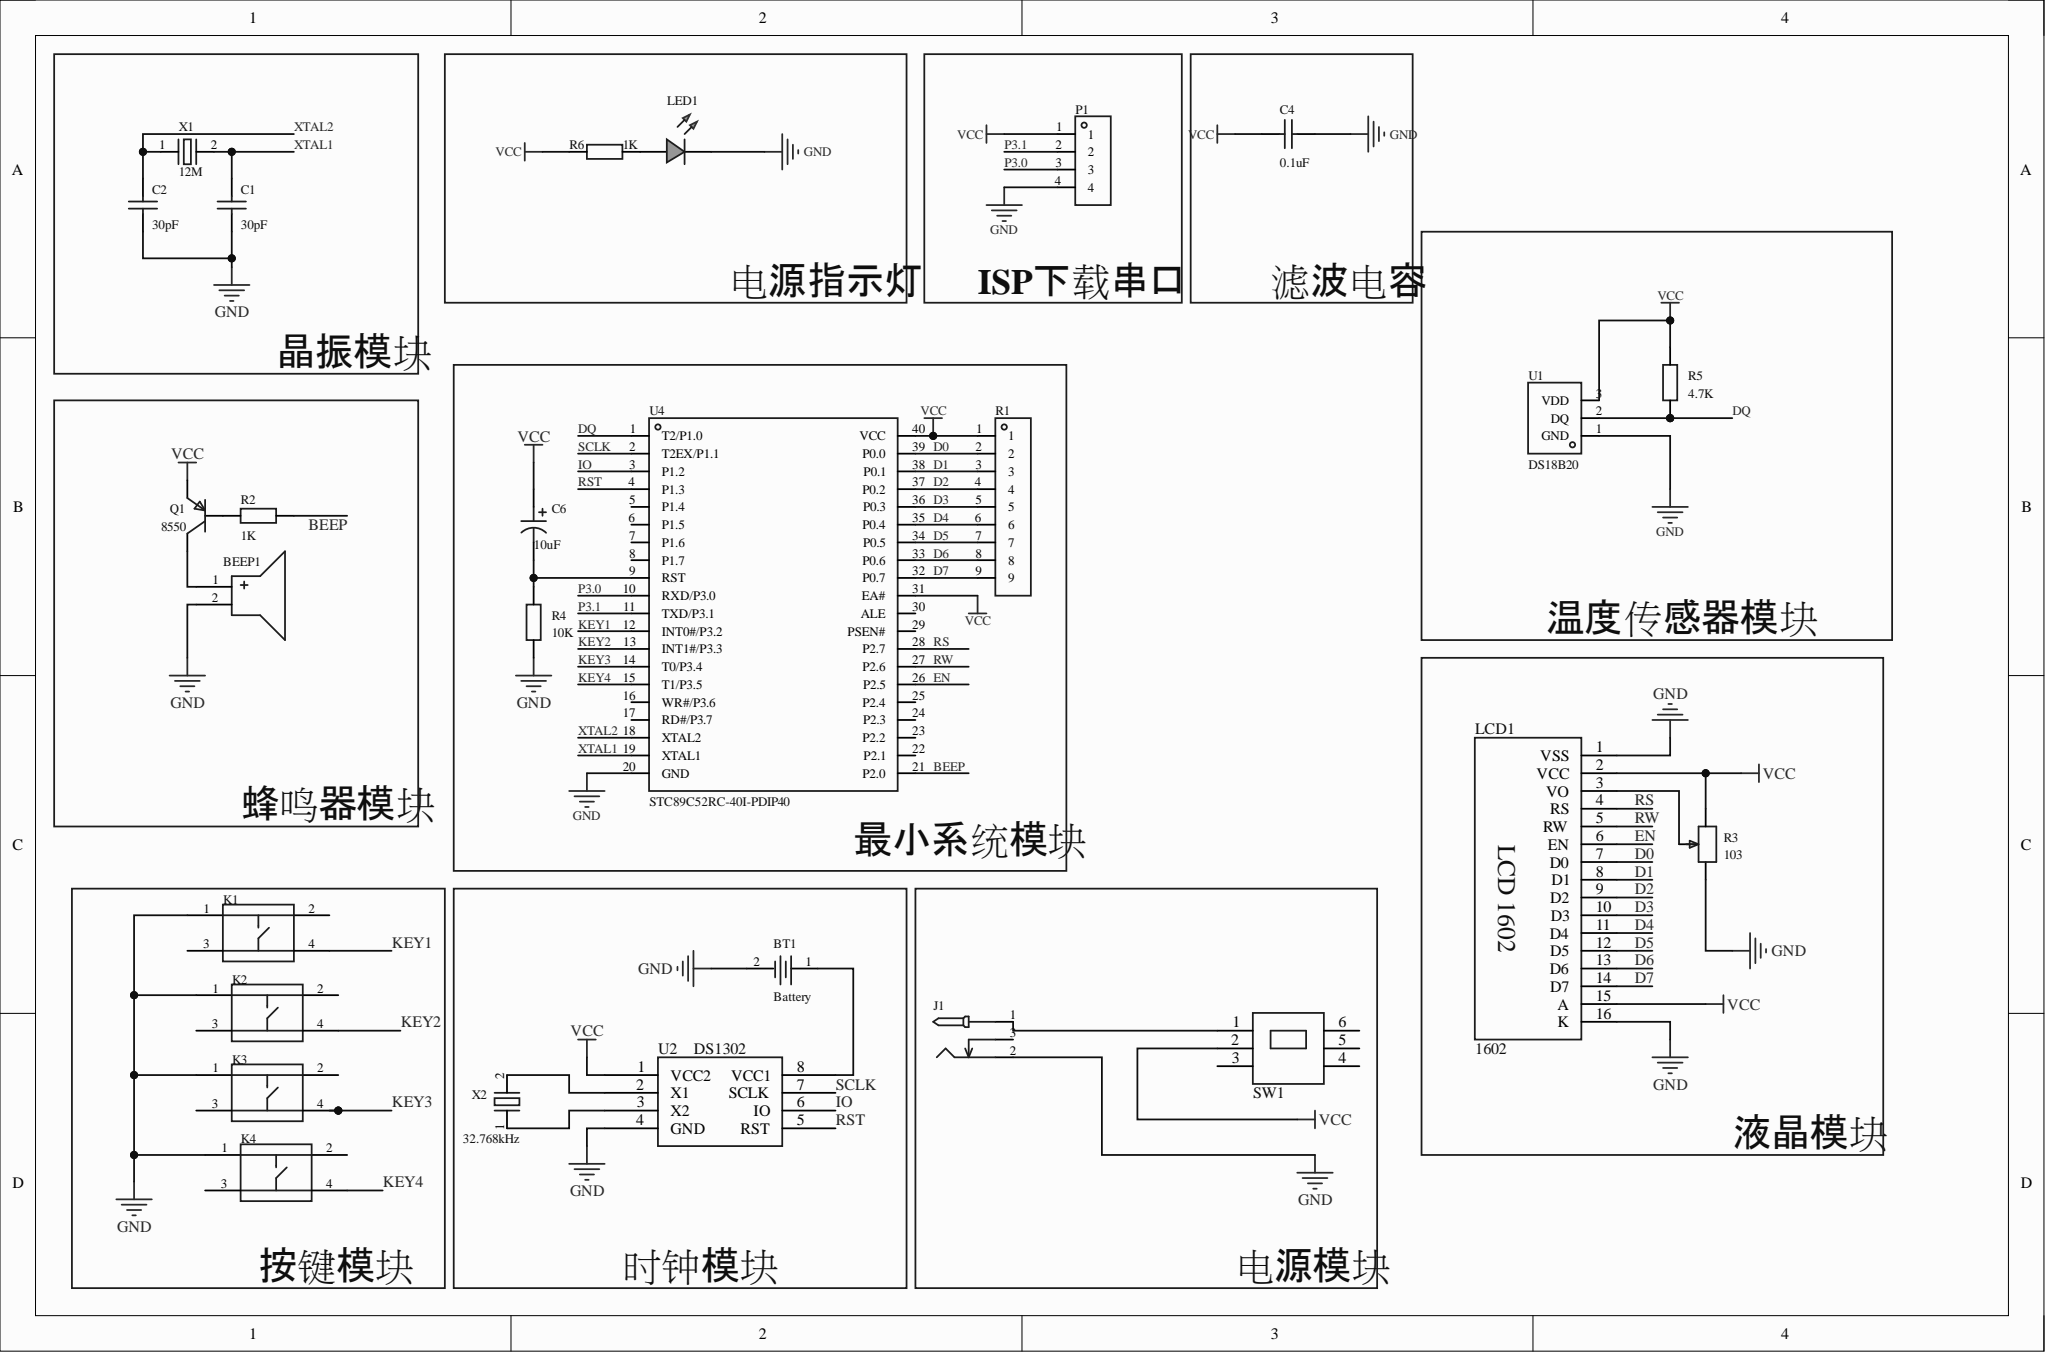Circuit board | Altium Designer | 27 parts | 35 nets
Bill of materials:
Comment,Description,Designator,Footprint,LibRef,Quantity
"","","BEEP1","BUZ-TH_BD12.0-P7.60-D0.6-FD","BZ-D12-L7_6","1"
"Battery","","BT1","BAT-TH_CR2032","Q&J CR2032 20-6*9_C9900112302","1"
"30pF","容值:-;额定电压:-;温度系数:-;","C1, C2","CAP-TH_L5.0-W4.0-P5.00-D1.0","瓷片电容47PF 3KV","2"
"0.1uF","容值:-;额定电压:-;温度系数:-;","C4","CAP-TH_L5.0-W4.0-P5.00-D1.0","瓷片电容47PF 3KV","1"
"10uF","","C6","CAP-TH_BD5.0-P2.00-D0.6-FD","10uF/25V-C5X11DIP","1"
"","","J1","DC-005_2.5","DC-005_2.5","1"
"","电路结构:单刀单掷;按钮形状:圆形按钮;作用力:2.5N;安装方式:直插;开关长度:6mm;开关宽度:6mm;开关高度:5mm;触点电流:50mA;额定电压:12V;带灯:-;工作寿命:10万次;","K1, K2, K3, K4","KEY-TH_4P-L6.0-W6.0-P4.50-LS6.50","K2-1102DP-C4SW-04","4"
"1602","","LCD1","HDR-M-2.54_1X16","1602_1","1"
"","","LED1","LED-TH_5mm","LED_TH-G_5mm","1"
"","","P1","HDR-TH_4P-P2.54-V-M","HDR-M_2.54_1x4P","1"
"8550","","Q1","S8550P_TO-92","S8550_TO_PNP","1"
"","","R1","SIP-9_L22.3-W3.2-P2.54_KA2284-SIP-9","HDR-M_2.54-1x9P","1"
"1K","","R2, R6","Res_1/4W","Res_AXIAL-1/4W","2"
"103","","R3","RES-ADJ-SMD_RM065-V1","RM065-V1-103","1"
"10K","","R4","Res_1/4W","Res_AXIAL-1/4W","1"
"4.7K","","R5","Res_1/4W","Res_AXIAL-1/4W","1"
"SWT","","SW1","SW-TH_6P-L8.5-W8.5-P2.50-LS5.5-BL-2","SWT_1","1"
"DS18B20","检测温度:-55℃~+125℃;精度:±0.4℃;接口类型:单总线;","U1","TO-92-3_L4.5-W3.5-P1.27-L","DS18B20","1"
"DS1302","","U2","DIP-8_L10.9-W6.4-P2.54-LS7.6-BL","DS1302","1"
"STC89C52RC-40I-PDIP40","CPU内核:51家族;CPU最大主频:-;","U4","DIP-40_L52.0-W13.7-P2.54-LS15.2-BL","STC89C52RC-40I-PDIP40","1"
"12M","晶振类型:直插晶振;频率:16MHz;常温频差:±20ppm;负载电容:12pF;频率稳定度:±30ppm;","X1","HC-49S_L11.5-W4.7-P4.88","SWXSBBCVE0-16","1"
"32.768kHz","频率:32.768kHz;常温频差:±20ppm;外接负载电容:12.5pF;频率稳定度(全温):-;","X2","XTAL2","AB15T-32.768KHZ","1"
Netlist (Protel format):
[
BEEP1
BUZ-TH_BD12.0-P7.60-D0.6-FD




]
[
BT1
BAT-TH_CR2032
Battery



]
[
C1
CAP-TH_L5.0-W4.0-P5.00-D1.0
30pF



]
[
C2
CAP-TH_L5.0-W4.0-P5.00-D1.0
30pF



]
[
C4
CAP-TH_L5.0-W4.0-P5.00-D1.0
0.1uF



]
[
C6
CAP-TH_BD5.0-P2.00-D0.6-FD
10uF



]
[
J1
DC-005_2.5




]
[
K1
KEY-TH_4P-L6.0-W6.0-P4.50-LS6.50




]
[
K2
KEY-TH_4P-L6.0-W6.0-P4.50-LS6.50




]
[
K3
KEY-TH_4P-L6.0-W6.0-P4.50-LS6.50




]
[
K4
KEY-TH_4P-L6.0-W6.0-P4.50-LS6.50




]
[
LCD1
HDR-M-2.54_1X16
1602



]
[
LED1
LED-TH_5mm




]
[
P1
HDR-TH_4P-P2.54-V-M




]
[
Q1
S8550P_TO-92
8550



]
[
R1
SIP-9_L22.3-W3.2-P2.54_KA2284-SIP-9




]
[
R2
Res_1/4W
1K



]
[
R3
RES-ADJ-SMD_RM065-V1
103



]
[
R4
Res_1/4W
10K



]
[
R5
Res_1/4W
4.7K



]
[
R6
Res_1/4W
1K



]
[
SW1
SW-TH_6P-L8.5-W8.5-P2.50-LS5.5-BL-2
SWT



]
[
U1
TO-92-3_L4.5-W3.5-P1.27-L
DS18B20



]
[
U2
DIP-8_L10.9-W6.4-P2.54-LS7.6-BL
DS1302



]
[
U4
DIP-40_L52.0-W13.7-P2.54-LS15.2-BL
STC89C52RC-40I-PDIP40



]
[
X1
HC-49S_L11.5-W4.7-P4.88
12M



]
[
X2
XTAL2
32.768kHz



]
(
XTAL2
C2-2
U4-18
X1-1
)
(
XTAL1
C1-2
U4-19
X1-2
)
(
VCC
C4-1
C6-1
LCD1-2
LCD1-15
P1-1
Q1-1
R1-1
R3-3
R5-2
R6-1
SW1-2
U1-3
U2-1
U4-31
U4-40
)
(
SCLK
U2-7
U4-2
)
(
RW
LCD1-5
U4-27
)
(
RST
U2-5
U4-4
)
(
RS
LCD1-4
U4-28
)
(
P3.1
P1-2
U4-11
)
(
P3.0
P1-3
U4-10
)
(
NetU2_3
U2-3
X2-1
)
(
NetU2_2
U2-2
X2-2
)
(
NetQ1_2
Q1-2
R2-1
)
(
NetLED1_1
LED1-1
R6-2
)
(
NetLCD1_3
LCD1-3
R3-2
)
(
NetJ1_1
J1-1
SW1-1
)
(
NetC6_2
C6-2
R4-2
U4-9
)
(
NetBT1_1
BT1-1
U2-8
)
(
NetBEEP1_1
BEEP1-1
Q1-3
)
(
KEY4
K4-4
U4-15
)
(
KEY3
K3-4
U4-14
)
(
KEY2
K2-4
U4-13
)
(
KEY1
K1-4
U4-12
)
(
IO
U2-6
U4-3
)
(
GND
BEEP1-2
BT1-2
C1-1
C2-1
C4-2
J1-2
K1-1
K2-1
K3-1
K4-1
LCD1-1
LCD1-16
LED1-2
P1-4
R3-1
R4-1
U1-1
U2-4
U4-20
)
(
EN
LCD1-6
U4-26
)
(
DQ
R5-1
U1-2
U4-1
)
(
D7
LCD1-14
R1-9
U4-32
)
(
D6
LCD1-13
R1-8
U4-33
)
(
D5
LCD1-12
R1-7
U4-34
)
(
D4
LCD1-11
R1-6
U4-35
)
(
D3
LCD1-10
R1-5
U4-36
)
(
D2
LCD1-9
R1-4
U4-37
)
(
D1
LCD1-8
R1-3
U4-38
)
(
D0
LCD1-7
R1-2
U4-39
)
(
BEEP
R2-2
U4-21
)